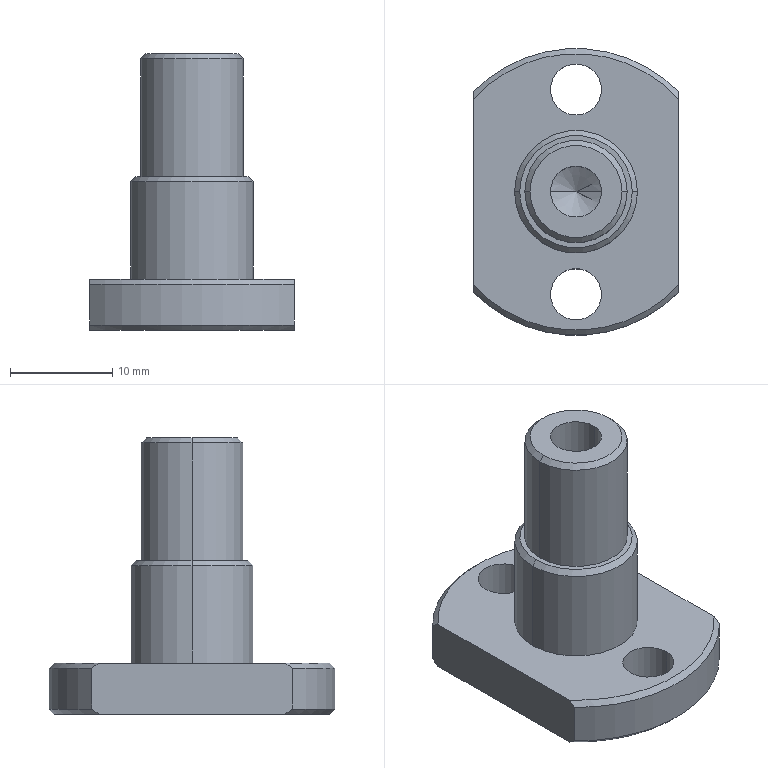Part | SolidWorks | features ICE 3, Chamfer 2, HoleWzd 2, Extrusion 1 | 1 solid | 28 faces | box 20 x 28 x 27 mm | volume 4092 mm3 | cylinder 12 | cone 10 | plane 6 | commonest cylinder face diameters 5 x6 10 x2 12 x2 28 x2
STEP:
#1=CARTESIAN_POINT('',(4.5,0.,22.));
#2=VERTEX_POINT('',#1);
#3=CARTESIAN_POINT('',(-4.5,0.,22.));
#4=VERTEX_POINT('',#3);
#5=CARTESIAN_POINT('',(0.,0.,22.));
#6=DIRECTION('',(0.,0.,1.));
#7=DIRECTION('',(1.,0.,0.));
#8=AXIS2_PLACEMENT_3D('',#5,#6,#7);
#9=CIRCLE('',#8,4.5);
#10=EDGE_CURVE('',#2,#4,#9,.T.);
#11=ORIENTED_EDGE('',*,*,#10,.F.);
#12=CARTESIAN_POINT('',(5.,0.,21.5));
#13=VERTEX_POINT('',#12);
#14=CARTESIAN_POINT('',(4.5,0.,22.));
#15=DIRECTION('',(0.7071,0.,-0.7071));
#16=VECTOR('',#15,1000.);
#17=LINE('',#14,#16);
#18=EDGE_CURVE('',#2,#13,#17,.T.);
#19=ORIENTED_EDGE('',*,*,#18,.T.);
#20=CARTESIAN_POINT('',(-5.,0.,21.5));
#21=VERTEX_POINT('',#20);
#22=CARTESIAN_POINT('',(0.,0.,21.5));
#23=DIRECTION('',(0.,0.,-1.));
#24=DIRECTION('',(1.,0.,0.));
#25=AXIS2_PLACEMENT_3D('',#22,#23,#24);
#26=CIRCLE('',#25,5.);
#27=EDGE_CURVE('',#21,#13,#26,.T.);
#28=ORIENTED_EDGE('',*,*,#27,.F.);
#29=CARTESIAN_POINT('',(-4.5,0.,22.));
#30=DIRECTION('',(-0.7071,0.,-0.7071));
#31=VECTOR('',#30,1000.);
#32=LINE('',#29,#31);
#33=EDGE_CURVE('',#4,#21,#32,.T.);
#34=ORIENTED_EDGE('',*,*,#33,.F.);
#35=EDGE_LOOP('',(#11,#19,#28,#34));
#36=FACE_OUTER_BOUND('',#35,.T.);
#37=CARTESIAN_POINT('',(0.,0.,22.));
#38=DIRECTION('',(0.,0.,-1.));
#39=DIRECTION('',(-1.,0.,0.));
#40=AXIS2_PLACEMENT_3D('',#37,#38,#39);
#41=CONICAL_SURFACE('',#40,4.5,0.7854);
#42=ADVANCED_FACE('',(#36),#41,.T.);
#43=CARTESIAN_POINT('',(5.5,0.,10.));
#44=VERTEX_POINT('',#43);
#45=CARTESIAN_POINT('',(-5.5,0.,10.));
#46=VERTEX_POINT('',#45);
#47=CARTESIAN_POINT('',(0.,0.,10.));
#48=DIRECTION('',(0.,0.,1.));
#49=DIRECTION('',(-1.,0.,0.));
#50=AXIS2_PLACEMENT_3D('',#47,#48,#49);
#51=CIRCLE('',#50,5.5);
#52=EDGE_CURVE('',#44,#46,#51,.T.);
#53=ORIENTED_EDGE('',*,*,#52,.F.);
#54=CARTESIAN_POINT('',(6.,0.,9.5));
#55=VERTEX_POINT('',#54);
#56=CARTESIAN_POINT('',(6.,0.,9.5));
#57=DIRECTION('',(0.7071,0.,-0.7071));
#58=VECTOR('',#57,1000.);
#59=LINE('',#56,#58);
#60=EDGE_CURVE('',#44,#55,#59,.T.);
#61=ORIENTED_EDGE('',*,*,#60,.T.);
#62=CARTESIAN_POINT('',(-6.,0.,9.5));
#63=VERTEX_POINT('',#62);
#64=CARTESIAN_POINT('',(0.,0.,9.5));
#65=DIRECTION('',(0.,0.,-1.));
#66=DIRECTION('',(-1.,0.,0.));
#67=AXIS2_PLACEMENT_3D('',#64,#65,#66);
#68=CIRCLE('',#67,6.);
#69=EDGE_CURVE('',#63,#55,#68,.T.);
#70=ORIENTED_EDGE('',*,*,#69,.F.);
#71=CARTESIAN_POINT('',(-6.,0.,9.5));
#72=DIRECTION('',(-0.7071,0.,-0.7071));
#73=VECTOR('',#72,1000.);
#74=LINE('',#71,#73);
#75=EDGE_CURVE('',#46,#63,#74,.T.);
#76=ORIENTED_EDGE('',*,*,#75,.F.);
#77=EDGE_LOOP('',(#53,#61,#70,#76));
#78=FACE_OUTER_BOUND('',#77,.T.);
#79=CARTESIAN_POINT('',(0.,0.,9.5));
#80=DIRECTION('',(0.,0.,-1.));
#81=DIRECTION('',(-1.,0.,0.));
#82=AXIS2_PLACEMENT_3D('',#79,#80,#81);
#83=CONICAL_SURFACE('',#82,6.,0.7854);
#84=ADVANCED_FACE('',(#78),#83,.T.);
#85=CARTESIAN_POINT('',(-2.5,0.,7.));
#86=VERTEX_POINT('',#85);
#87=CARTESIAN_POINT('',(2.5,0.,7.));
#88=VERTEX_POINT('',#87);
#89=CARTESIAN_POINT('',(0.,0.,7.));
#90=DIRECTION('',(0.,0.,1.));
#91=DIRECTION('',(1.,0.,0.));
#92=AXIS2_PLACEMENT_3D('',#89,#90,#91);
#93=CIRCLE('',#92,2.5);
#94=EDGE_CURVE('',#86,#88,#93,.T.);
#95=ORIENTED_EDGE('',*,*,#94,.F.);
#96=CARTESIAN_POINT('',(-2.5,0.,22.));
#97=VERTEX_POINT('',#96);
#98=CARTESIAN_POINT('',(-2.5,0.,22.));
#99=DIRECTION('',(0.,0.,1.));
#100=VECTOR('',#99,1000.);
#101=LINE('',#98,#100);
#102=EDGE_CURVE('',#86,#97,#101,.T.);
#103=ORIENTED_EDGE('',*,*,#102,.T.);
#104=CARTESIAN_POINT('',(2.5,0.,22.));
#105=VERTEX_POINT('',#104);
#106=CARTESIAN_POINT('',(0.,0.,22.));
#107=DIRECTION('',(0.,0.,1.));
#108=DIRECTION('',(1.,0.,0.));
#109=AXIS2_PLACEMENT_3D('',#106,#107,#108);
#110=CIRCLE('',#109,2.5);
#111=EDGE_CURVE('',#97,#105,#110,.T.);
#112=ORIENTED_EDGE('',*,*,#111,.T.);
#113=CARTESIAN_POINT('',(2.5,0.,22.));
#114=DIRECTION('',(0.,0.,1.));
#115=VECTOR('',#114,1000.);
#116=LINE('',#113,#115);
#117=EDGE_CURVE('',#88,#105,#116,.T.);
#118=ORIENTED_EDGE('',*,*,#117,.F.);
#119=EDGE_LOOP('',(#95,#103,#112,#118));
#120=FACE_OUTER_BOUND('',#119,.T.);
#121=CARTESIAN_POINT('',(0.,0.,22.));
#122=DIRECTION('',(0.,0.,1.));
#123=DIRECTION('',(1.,0.,0.));
#124=AXIS2_PLACEMENT_3D('',#121,#122,#123);
#125=CYLINDRICAL_SURFACE('',#124,2.5);
#126=ADVANCED_FACE('',(#120),#125,.F.);
#127=CARTESIAN_POINT('',(0.,0.,5.498));
#128=VERTEX_POINT('',#127);
#129=CARTESIAN_POINT('',(2.5,0.,7.));
#130=DIRECTION('',(0.8572,0.,0.515));
#131=VECTOR('',#130,1000.);
#132=LINE('',#129,#131);
#133=EDGE_CURVE('',#128,#88,#132,.T.);
#134=ORIENTED_EDGE('',*,*,#133,.F.);
#135=CARTESIAN_POINT('',(-2.5,0.,7.));
#136=DIRECTION('',(-0.8572,0.,0.515));
#137=VECTOR('',#136,1000.);
#138=LINE('',#135,#137);
#139=EDGE_CURVE('',#128,#86,#138,.T.);
#140=ORIENTED_EDGE('',*,*,#139,.T.);
#141=ORIENTED_EDGE('',*,*,#94,.T.);
#142=EDGE_LOOP('',(#134,#140,#141));
#143=FACE_OUTER_BOUND('',#142,.T.);
#144=CARTESIAN_POINT('',(0.,0.,7.));
#145=DIRECTION('',(0.,0.,1.));
#146=DIRECTION('',(1.,0.,0.));
#147=AXIS2_PLACEMENT_3D('',#144,#145,#146);
#148=CONICAL_SURFACE('',#147,2.5,1.03);
#149=ADVANCED_FACE('',(#143),#148,.F.);
#150=CARTESIAN_POINT('',(2.5,10.,-5.));
#151=VERTEX_POINT('',#150);
#152=CARTESIAN_POINT('',(-2.5,10.,-5.));
#153=VERTEX_POINT('',#152);
#154=CARTESIAN_POINT('',(0.,10.,-5.));
#155=DIRECTION('',(0.,0.,-1.));
#156=DIRECTION('',(-1.,0.,0.));
#157=AXIS2_PLACEMENT_3D('',#154,#155,#156);
#158=CIRCLE('',#157,2.5);
#159=EDGE_CURVE('',#151,#153,#158,.T.);
#160=ORIENTED_EDGE('',*,*,#159,.T.);
#161=CARTESIAN_POINT('',(-2.5,10.,0.));
#162=VERTEX_POINT('',#161);
#163=CARTESIAN_POINT('',(-2.5,10.,0.));
#164=DIRECTION('',(0.,0.,1.));
#165=VECTOR('',#164,1000.);
#166=LINE('',#163,#165);
#167=EDGE_CURVE('',#153,#162,#166,.T.);
#168=ORIENTED_EDGE('',*,*,#167,.T.);
#169=CARTESIAN_POINT('',(2.5,10.,0.));
#170=VERTEX_POINT('',#169);
#171=CARTESIAN_POINT('',(0.,10.,0.));
#172=DIRECTION('',(0.,0.,1.));
#173=DIRECTION('',(1.,0.,0.));
#174=AXIS2_PLACEMENT_3D('',#171,#172,#173);
#175=CIRCLE('',#174,2.5);
#176=EDGE_CURVE('',#162,#170,#175,.T.);
#177=ORIENTED_EDGE('',*,*,#176,.T.);
#178=CARTESIAN_POINT('',(2.5,10.,0.));
#179=DIRECTION('',(0.,0.,1.));
#180=VECTOR('',#179,1000.);
#181=LINE('',#178,#180);
#182=EDGE_CURVE('',#151,#170,#181,.T.);
#183=ORIENTED_EDGE('',*,*,#182,.F.);
#184=EDGE_LOOP('',(#160,#168,#177,#183));
#185=FACE_OUTER_BOUND('',#184,.T.);
#186=CARTESIAN_POINT('',(0.,10.,0.));
#187=DIRECTION('',(0.,0.,1.));
#188=DIRECTION('',(1.,0.,0.));
#189=AXIS2_PLACEMENT_3D('',#186,#187,#188);
#190=CYLINDRICAL_SURFACE('',#189,2.5);
#191=ADVANCED_FACE('',(#185),#190,.F.);
#192=CARTESIAN_POINT('',(2.5,-10.,-5.));
#193=VERTEX_POINT('',#192);
#194=CARTESIAN_POINT('',(-2.5,-10.,-5.));
#195=VERTEX_POINT('',#194);
#196=CARTESIAN_POINT('',(0.,-10.,-5.));
#197=DIRECTION('',(0.,0.,-1.));
#198=DIRECTION('',(-1.,0.,0.));
#199=AXIS2_PLACEMENT_3D('',#196,#197,#198);
#200=CIRCLE('',#199,2.5);
#201=EDGE_CURVE('',#193,#195,#200,.T.);
#202=ORIENTED_EDGE('',*,*,#201,.T.);
#203=CARTESIAN_POINT('',(-2.5,-10.,0.));
#204=VERTEX_POINT('',#203);
#205=CARTESIAN_POINT('',(-2.5,-10.,0.));
#206=DIRECTION('',(0.,0.,1.));
#207=VECTOR('',#206,1000.);
#208=LINE('',#205,#207);
#209=EDGE_CURVE('',#195,#204,#208,.T.);
#210=ORIENTED_EDGE('',*,*,#209,.T.);
#211=CARTESIAN_POINT('',(2.5,-10.,0.));
#212=VERTEX_POINT('',#211);
#213=CARTESIAN_POINT('',(0.,-10.,0.));
#214=DIRECTION('',(0.,0.,1.));
#215=DIRECTION('',(1.,0.,0.));
#216=AXIS2_PLACEMENT_3D('',#213,#214,#215);
#217=CIRCLE('',#216,2.5);
#218=EDGE_CURVE('',#204,#212,#217,.T.);
#219=ORIENTED_EDGE('',*,*,#218,.T.);
#220=CARTESIAN_POINT('',(2.5,-10.,0.));
#221=DIRECTION('',(0.,0.,1.));
#222=VECTOR('',#221,1000.);
#223=LINE('',#220,#222);
#224=EDGE_CURVE('',#193,#212,#223,.T.);
#225=ORIENTED_EDGE('',*,*,#224,.F.);
#226=EDGE_LOOP('',(#202,#210,#219,#225));
#227=FACE_OUTER_BOUND('',#226,.T.);
#228=CARTESIAN_POINT('',(0.,-10.,0.));
#229=DIRECTION('',(0.,0.,1.));
#230=DIRECTION('',(1.,0.,0.));
#231=AXIS2_PLACEMENT_3D('',#228,#229,#230);
#232=CYLINDRICAL_SURFACE('',#231,2.5);
#233=ADVANCED_FACE('',(#227),#232,.F.);
#234=ORIENTED_EDGE('',*,*,#69,.T.);
#235=CARTESIAN_POINT('',(6.,0.,0.));
#236=VERTEX_POINT('',#235);
#237=CARTESIAN_POINT('',(6.,0.,10.));
#238=DIRECTION('',(0.,0.,-1.));
#239=VECTOR('',#238,1000.);
#240=LINE('',#237,#239);
#241=EDGE_CURVE('',#55,#236,#240,.T.);
#242=ORIENTED_EDGE('',*,*,#241,.T.);
#243=CARTESIAN_POINT('',(-6.,0.,0.));
#244=VERTEX_POINT('',#243);
#245=CARTESIAN_POINT('',(0.,0.,0.));
#246=DIRECTION('',(0.,0.,-1.));
#247=DIRECTION('',(-1.,0.,0.));
#248=AXIS2_PLACEMENT_3D('',#245,#246,#247);
#249=CIRCLE('',#248,6.);
#250=EDGE_CURVE('',#244,#236,#249,.T.);
#251=ORIENTED_EDGE('',*,*,#250,.F.);
#252=CARTESIAN_POINT('',(-6.,0.,10.));
#253=DIRECTION('',(0.,0.,-1.));
#254=VECTOR('',#253,1000.);
#255=LINE('',#252,#254);
#256=EDGE_CURVE('',#63,#244,#255,.T.);
#257=ORIENTED_EDGE('',*,*,#256,.F.);
#258=EDGE_LOOP('',(#234,#242,#251,#257));
#259=FACE_OUTER_BOUND('',#258,.T.);
#260=CARTESIAN_POINT('',(0.,0.,10.));
#261=DIRECTION('',(0.,0.,-1.));
#262=DIRECTION('',(-1.,0.,0.));
#263=AXIS2_PLACEMENT_3D('',#260,#261,#262);
#264=CYLINDRICAL_SURFACE('',#263,6.);
#265=ADVANCED_FACE('',(#259),#264,.T.);
#266=ORIENTED_EDGE('',*,*,#27,.T.);
#267=CARTESIAN_POINT('',(5.,0.,10.));
#268=VERTEX_POINT('',#267);
#269=CARTESIAN_POINT('',(5.,0.,22.));
#270=DIRECTION('',(0.,0.,-1.));
#271=VECTOR('',#270,1000.);
#272=LINE('',#269,#271);
#273=EDGE_CURVE('',#13,#268,#272,.T.);
#274=ORIENTED_EDGE('',*,*,#273,.T.);
#275=CARTESIAN_POINT('',(-5.,0.,10.));
#276=VERTEX_POINT('',#275);
#277=CARTESIAN_POINT('',(0.,0.,10.));
#278=DIRECTION('',(0.,0.,-1.));
#279=DIRECTION('',(-1.,0.,0.));
#280=AXIS2_PLACEMENT_3D('',#277,#278,#279);
#281=CIRCLE('',#280,5.);
#282=EDGE_CURVE('',#276,#268,#281,.T.);
#283=ORIENTED_EDGE('',*,*,#282,.F.);
#284=CARTESIAN_POINT('',(-5.,0.,22.));
#285=DIRECTION('',(0.,0.,-1.));
#286=VECTOR('',#285,1000.);
#287=LINE('',#284,#286);
#288=EDGE_CURVE('',#21,#276,#287,.T.);
#289=ORIENTED_EDGE('',*,*,#288,.F.);
#290=EDGE_LOOP('',(#266,#274,#283,#289));
#291=FACE_OUTER_BOUND('',#290,.T.);
#292=CARTESIAN_POINT('',(0.,0.,22.));
#293=DIRECTION('',(0.,0.,-1.));
#294=DIRECTION('',(-1.,0.,0.));
#295=AXIS2_PLACEMENT_3D('',#292,#293,#294);
#296=CYLINDRICAL_SURFACE('',#295,5.);
#297=ADVANCED_FACE('',(#291),#296,.T.);
#298=CARTESIAN_POINT('',(10.,9.798,-4.5));
#299=VERTEX_POINT('',#298);
#300=CARTESIAN_POINT('',(10.,9.798,-0.5));
#301=VERTEX_POINT('',#300);
#302=CARTESIAN_POINT('',(10.,9.798,-5.));
#303=DIRECTION('',(0.,0.,1.));
#304=VECTOR('',#303,1000.);
#305=LINE('',#302,#304);
#306=EDGE_CURVE('',#299,#301,#305,.T.);
#307=ORIENTED_EDGE('',*,*,#306,.F.);
#308=CARTESIAN_POINT('',(-10.,9.798,-4.5));
#309=VERTEX_POINT('',#308);
#310=CARTESIAN_POINT('',(0.,0.,-4.5));
#311=DIRECTION('',(0.,0.,1.));
#312=DIRECTION('',(-1.,0.,0.));
#313=AXIS2_PLACEMENT_3D('',#310,#311,#312);
#314=CIRCLE('',#313,14.);
#315=EDGE_CURVE('',#299,#309,#314,.T.);
#316=ORIENTED_EDGE('',*,*,#315,.T.);
#317=CARTESIAN_POINT('',(-10.,9.798,-0.5));
#318=VERTEX_POINT('',#317);
#319=CARTESIAN_POINT('',(-10.,9.798,-5.));
#320=DIRECTION('',(0.,0.,-1.));
#321=VECTOR('',#320,1000.);
#322=LINE('',#319,#321);
#323=EDGE_CURVE('',#318,#309,#322,.T.);
#324=ORIENTED_EDGE('',*,*,#323,.F.);
#325=CARTESIAN_POINT('',(0.,0.,-0.5));
#326=DIRECTION('',(0.,0.,-1.));
#327=DIRECTION('',(-1.,0.,0.));
#328=AXIS2_PLACEMENT_3D('',#325,#326,#327);
#329=CIRCLE('',#328,14.);
#330=EDGE_CURVE('',#318,#301,#329,.T.);
#331=ORIENTED_EDGE('',*,*,#330,.T.);
#332=EDGE_LOOP('',(#307,#316,#324,#331));
#333=FACE_OUTER_BOUND('',#332,.T.);
#334=CARTESIAN_POINT('',(0.,0.,-5.));
#335=DIRECTION('',(0.,0.,1.));
#336=DIRECTION('',(1.,0.,0.));
#337=AXIS2_PLACEMENT_3D('',#334,#335,#336);
#338=CYLINDRICAL_SURFACE('',#337,14.);
#339=ADVANCED_FACE('',(#333),#338,.T.);
#340=CARTESIAN_POINT('',(-10.,-9.798,-4.5));
#341=VERTEX_POINT('',#340);
#342=CARTESIAN_POINT('',(-10.,-9.798,-0.5));
#343=VERTEX_POINT('',#342);
#344=CARTESIAN_POINT('',(-10.,-9.798,-5.));
#345=DIRECTION('',(0.,0.,1.));
#346=VECTOR('',#345,1000.);
#347=LINE('',#344,#346);
#348=EDGE_CURVE('',#341,#343,#347,.T.);
#349=ORIENTED_EDGE('',*,*,#348,.F.);
#350=CARTESIAN_POINT('',(10.,-9.798,-4.5));
#351=VERTEX_POINT('',#350);
#352=CARTESIAN_POINT('',(0.,0.,-4.5));
#353=DIRECTION('',(0.,0.,1.));
#354=DIRECTION('',(-1.,0.,0.));
#355=AXIS2_PLACEMENT_3D('',#352,#353,#354);
#356=CIRCLE('',#355,14.);
#357=EDGE_CURVE('',#341,#351,#356,.T.);
#358=ORIENTED_EDGE('',*,*,#357,.T.);
#359=CARTESIAN_POINT('',(10.,-9.798,-0.5));
#360=VERTEX_POINT('',#359);
#361=CARTESIAN_POINT('',(10.,-9.798,-5.));
#362=DIRECTION('',(0.,0.,-1.));
#363=VECTOR('',#362,1000.);
#364=LINE('',#361,#363);
#365=EDGE_CURVE('',#360,#351,#364,.T.);
#366=ORIENTED_EDGE('',*,*,#365,.F.);
#367=CARTESIAN_POINT('',(0.,0.,-0.5));
#368=DIRECTION('',(0.,0.,-1.));
#369=DIRECTION('',(-1.,0.,0.));
#370=AXIS2_PLACEMENT_3D('',#367,#368,#369);
#371=CIRCLE('',#370,14.);
#372=EDGE_CURVE('',#360,#343,#371,.T.);
#373=ORIENTED_EDGE('',*,*,#372,.T.);
#374=EDGE_LOOP('',(#349,#358,#366,#373));
#375=FACE_OUTER_BOUND('',#374,.T.);
#376=CARTESIAN_POINT('',(0.,0.,-5.));
#377=DIRECTION('',(0.,0.,1.));
#378=DIRECTION('',(1.,0.,0.));
#379=AXIS2_PLACEMENT_3D('',#376,#377,#378);
#380=CYLINDRICAL_SURFACE('',#379,14.);
#381=ADVANCED_FACE('',(#375),#380,.T.);
#382=ORIENTED_EDGE('',*,*,#159,.F.);
#383=CARTESIAN_POINT('',(0.,10.,-5.));
#384=DIRECTION('',(0.,0.,-1.));
#385=DIRECTION('',(-1.,0.,0.));
#386=AXIS2_PLACEMENT_3D('',#383,#384,#385);
#387=CIRCLE('',#386,2.5);
#388=EDGE_CURVE('',#153,#151,#387,.T.);
#389=ORIENTED_EDGE('',*,*,#388,.F.);
#390=EDGE_LOOP('',(#382,#389));
#391=FACE_BOUND('',#390,.T.);
#392=ORIENTED_EDGE('',*,*,#201,.F.);
#393=CARTESIAN_POINT('',(0.,-10.,-5.));
#394=DIRECTION('',(0.,0.,-1.));
#395=DIRECTION('',(-1.,0.,0.));
#396=AXIS2_PLACEMENT_3D('',#393,#394,#395);
#397=CIRCLE('',#396,2.5);
#398=EDGE_CURVE('',#195,#193,#397,.T.);
#399=ORIENTED_EDGE('',*,*,#398,.F.);
#400=EDGE_LOOP('',(#392,#399));
#401=FACE_BOUND('',#400,.T.);
#402=CARTESIAN_POINT('',(10.,9.069,-5.));
#403=VERTEX_POINT('',#402);
#404=CARTESIAN_POINT('',(10.,-9.069,-5.));
#405=VERTEX_POINT('',#404);
#406=CARTESIAN_POINT('',(10.,18.644,-5.));
#407=DIRECTION('',(0.,-1.,0.));
#408=VECTOR('',#407,1000.);
#409=LINE('',#406,#408);
#410=EDGE_CURVE('',#403,#405,#409,.T.);
#411=ORIENTED_EDGE('',*,*,#410,.T.);
#412=CARTESIAN_POINT('',(-10.,-9.069,-5.));
#413=VERTEX_POINT('',#412);
#414=CARTESIAN_POINT('',(0.,0.,-5.));
#415=DIRECTION('',(0.,0.,-1.));
#416=DIRECTION('',(-1.,0.,0.));
#417=AXIS2_PLACEMENT_3D('',#414,#415,#416);
#418=CIRCLE('',#417,13.5);
#419=EDGE_CURVE('',#405,#413,#418,.T.);
#420=ORIENTED_EDGE('',*,*,#419,.T.);
#421=CARTESIAN_POINT('',(-10.,9.069,-5.));
#422=VERTEX_POINT('',#421);
#423=CARTESIAN_POINT('',(-10.,18.644,-5.));
#424=DIRECTION('',(0.,1.,0.));
#425=VECTOR('',#424,1000.);
#426=LINE('',#423,#425);
#427=EDGE_CURVE('',#413,#422,#426,.T.);
#428=ORIENTED_EDGE('',*,*,#427,.T.);
#429=CARTESIAN_POINT('',(0.,0.,-5.));
#430=DIRECTION('',(0.,0.,-1.));
#431=DIRECTION('',(-1.,0.,0.));
#432=AXIS2_PLACEMENT_3D('',#429,#430,#431);
#433=CIRCLE('',#432,13.5);
#434=EDGE_CURVE('',#422,#403,#433,.T.);
#435=ORIENTED_EDGE('',*,*,#434,.T.);
#436=EDGE_LOOP('',(#411,#420,#428,#435));
#437=FACE_OUTER_BOUND('',#436,.T.);
#438=CARTESIAN_POINT('',(0.,0.,-5.));
#439=DIRECTION('',(0.,0.,-1.));
#440=DIRECTION('',(-1.,0.,0.));
#441=AXIS2_PLACEMENT_3D('',#438,#439,#440);
#442=PLANE('',#441);
#443=ADVANCED_FACE('',(#391,#401,#437),#442,.T.);
#444=CARTESIAN_POINT('',(0.,10.,0.));
#445=DIRECTION('',(0.,0.,1.));
#446=DIRECTION('',(1.,0.,0.));
#447=AXIS2_PLACEMENT_3D('',#444,#445,#446);
#448=CIRCLE('',#447,2.5);
#449=EDGE_CURVE('',#170,#162,#448,.T.);
#450=ORIENTED_EDGE('',*,*,#449,.F.);
#451=ORIENTED_EDGE('',*,*,#176,.F.);
#452=EDGE_LOOP('',(#450,#451));
#453=FACE_BOUND('',#452,.T.);
#454=CARTESIAN_POINT('',(0.,-10.,0.));
#455=DIRECTION('',(0.,0.,1.));
#456=DIRECTION('',(1.,0.,0.));
#457=AXIS2_PLACEMENT_3D('',#454,#455,#456);
#458=CIRCLE('',#457,2.5);
#459=EDGE_CURVE('',#212,#204,#458,.T.);
#460=ORIENTED_EDGE('',*,*,#459,.F.);
#461=ORIENTED_EDGE('',*,*,#218,.F.);
#462=EDGE_LOOP('',(#460,#461));
#463=FACE_BOUND('',#462,.T.);
#464=ORIENTED_EDGE('',*,*,#250,.T.);
#465=CARTESIAN_POINT('',(0.,0.,0.));
#466=DIRECTION('',(0.,0.,-1.));
#467=DIRECTION('',(-1.,0.,0.));
#468=AXIS2_PLACEMENT_3D('',#465,#466,#467);
#469=CIRCLE('',#468,6.);
#470=EDGE_CURVE('',#236,#244,#469,.T.);
#471=ORIENTED_EDGE('',*,*,#470,.T.);
#472=EDGE_LOOP('',(#464,#471));
#473=FACE_BOUND('',#472,.T.);
#474=CARTESIAN_POINT('',(10.,9.069,0.));
#475=VERTEX_POINT('',#474);
#476=CARTESIAN_POINT('',(10.,-9.069,0.));
#477=VERTEX_POINT('',#476);
#478=CARTESIAN_POINT('',(10.,0.,0.));
#479=DIRECTION('',(0.,-1.,0.));
#480=VECTOR('',#479,1000.);
#481=LINE('',#478,#480);
#482=EDGE_CURVE('',#475,#477,#481,.T.);
#483=ORIENTED_EDGE('',*,*,#482,.F.);
#484=CARTESIAN_POINT('',(-10.,9.069,0.));
#485=VERTEX_POINT('',#484);
#486=CARTESIAN_POINT('',(0.,0.,0.));
#487=DIRECTION('',(0.,0.,1.));
#488=DIRECTION('',(-1.,0.,0.));
#489=AXIS2_PLACEMENT_3D('',#486,#487,#488);
#490=CIRCLE('',#489,13.5);
#491=EDGE_CURVE('',#475,#485,#490,.T.);
#492=ORIENTED_EDGE('',*,*,#491,.T.);
#493=CARTESIAN_POINT('',(-10.,-9.069,0.));
#494=VERTEX_POINT('',#493);
#495=CARTESIAN_POINT('',(-10.,0.,0.));
#496=DIRECTION('',(0.,1.,0.));
#497=VECTOR('',#496,1000.);
#498=LINE('',#495,#497);
#499=EDGE_CURVE('',#494,#485,#498,.T.);
#500=ORIENTED_EDGE('',*,*,#499,.F.);
#501=CARTESIAN_POINT('',(0.,0.,0.));
#502=DIRECTION('',(0.,0.,1.));
#503=DIRECTION('',(-1.,0.,0.));
#504=AXIS2_PLACEMENT_3D('',#501,#502,#503);
#505=CIRCLE('',#504,13.5);
#506=EDGE_CURVE('',#494,#477,#505,.T.);
#507=ORIENTED_EDGE('',*,*,#506,.T.);
#508=EDGE_LOOP('',(#483,#492,#500,#507));
#509=FACE_OUTER_BOUND('',#508,.T.);
#510=CARTESIAN_POINT('',(0.,0.,0.));
#511=DIRECTION('',(0.,0.,-1.));
#512=DIRECTION('',(-1.,0.,0.));
#513=AXIS2_PLACEMENT_3D('',#510,#511,#512);
#514=PLANE('',#513);
#515=ADVANCED_FACE('',(#453,#463,#473,#509),#514,.F.);
#516=ORIENTED_EDGE('',*,*,#273,.F.);
#517=CARTESIAN_POINT('',(0.,0.,21.5));
#518=DIRECTION('',(0.,0.,-1.));
#519=DIRECTION('',(1.,0.,0.));
#520=AXIS2_PLACEMENT_3D('',#517,#518,#519);
#521=CIRCLE('',#520,5.);
#522=EDGE_CURVE('',#13,#21,#521,.T.);
#523=ORIENTED_EDGE('',*,*,#522,.T.);
#524=ORIENTED_EDGE('',*,*,#288,.T.);
#525=CARTESIAN_POINT('',(0.,0.,10.));
#526=DIRECTION('',(0.,0.,-1.));
#527=DIRECTION('',(-1.,0.,0.));
#528=AXIS2_PLACEMENT_3D('',#525,#526,#527);
#529=CIRCLE('',#528,5.);
#530=EDGE_CURVE('',#268,#276,#529,.T.);
#531=ORIENTED_EDGE('',*,*,#530,.F.);
#532=EDGE_LOOP('',(#516,#523,#524,#531));
#533=FACE_OUTER_BOUND('',#532,.T.);
#534=CARTESIAN_POINT('',(0.,0.,22.));
#535=DIRECTION('',(0.,0.,-1.));
#536=DIRECTION('',(-1.,0.,0.));
#537=AXIS2_PLACEMENT_3D('',#534,#535,#536);
#538=CYLINDRICAL_SURFACE('',#537,5.);
#539=ADVANCED_FACE('',(#533),#538,.T.);
#540=CARTESIAN_POINT('',(0.,0.,22.));
#541=DIRECTION('',(0.,0.,1.));
#542=DIRECTION('',(1.,0.,0.));
#543=AXIS2_PLACEMENT_3D('',#540,#541,#542);
#544=CIRCLE('',#543,4.5);
#545=EDGE_CURVE('',#4,#2,#544,.T.);
#546=ORIENTED_EDGE('',*,*,#545,.T.);
#547=ORIENTED_EDGE('',*,*,#10,.T.);
#548=EDGE_LOOP('',(#546,#547));
#549=FACE_OUTER_BOUND('',#548,.T.);
#550=CARTESIAN_POINT('',(0.,0.,22.));
#551=DIRECTION('',(0.,0.,1.));
#552=DIRECTION('',(1.,0.,0.));
#553=AXIS2_PLACEMENT_3D('',#550,#551,#552);
#554=CIRCLE('',#553,2.5);
#555=EDGE_CURVE('',#105,#97,#554,.T.);
#556=ORIENTED_EDGE('',*,*,#555,.F.);
#557=ORIENTED_EDGE('',*,*,#111,.F.);
#558=EDGE_LOOP('',(#556,#557));
#559=FACE_BOUND('',#558,.T.);
#560=CARTESIAN_POINT('',(0.,0.,22.));
#561=DIRECTION('',(0.,0.,1.));
#562=DIRECTION('',(1.,0.,0.));
#563=AXIS2_PLACEMENT_3D('',#560,#561,#562);
#564=PLANE('',#563);
#565=ADVANCED_FACE('',(#549,#559),#564,.T.);
#566=CARTESIAN_POINT('',(0.,0.,10.));
#567=DIRECTION('',(0.,0.,1.));
#568=DIRECTION('',(-1.,0.,0.));
#569=AXIS2_PLACEMENT_3D('',#566,#567,#568);
#570=CIRCLE('',#569,5.5);
#571=EDGE_CURVE('',#46,#44,#570,.T.);
#572=ORIENTED_EDGE('',*,*,#571,.T.);
#573=ORIENTED_EDGE('',*,*,#52,.T.);
#574=EDGE_LOOP('',(#572,#573));
#575=FACE_OUTER_BOUND('',#574,.T.);
#576=ORIENTED_EDGE('',*,*,#282,.T.);
#577=ORIENTED_EDGE('',*,*,#530,.T.);
#578=EDGE_LOOP('',(#576,#577));
#579=FACE_BOUND('',#578,.T.);
#580=CARTESIAN_POINT('',(0.,0.,10.));
#581=DIRECTION('',(0.,0.,-1.));
#582=DIRECTION('',(-1.,0.,0.));
#583=AXIS2_PLACEMENT_3D('',#580,#581,#582);
#584=PLANE('',#583);
#585=ADVANCED_FACE('',(#575,#579),#584,.F.);
#586=ORIENTED_EDGE('',*,*,#241,.F.);
#587=CARTESIAN_POINT('',(0.,0.,9.5));
#588=DIRECTION('',(0.,0.,-1.));
#589=DIRECTION('',(-1.,0.,0.));
#590=AXIS2_PLACEMENT_3D('',#587,#588,#589);
#591=CIRCLE('',#590,6.);
#592=EDGE_CURVE('',#55,#63,#591,.T.);
#593=ORIENTED_EDGE('',*,*,#592,.T.);
#594=ORIENTED_EDGE('',*,*,#256,.T.);
#595=ORIENTED_EDGE('',*,*,#470,.F.);
#596=EDGE_LOOP('',(#586,#593,#594,#595));
#597=FACE_OUTER_BOUND('',#596,.T.);
#598=CARTESIAN_POINT('',(0.,0.,10.));
#599=DIRECTION('',(0.,0.,-1.));
#600=DIRECTION('',(-1.,0.,0.));
#601=AXIS2_PLACEMENT_3D('',#598,#599,#600);
#602=CYLINDRICAL_SURFACE('',#601,6.);
#603=ADVANCED_FACE('',(#597),#602,.T.);
#604=ORIENTED_EDGE('',*,*,#427,.F.);
#605=CARTESIAN_POINT('',(-10.,-9.069,-5.));
#606=CARTESIAN_POINT('',(-10.,-9.314,-4.836));
#607=CARTESIAN_POINT('',(-10.,-9.557,-4.669));
#608=CARTESIAN_POINT('',(-10.,-9.798,-4.5));
#609=B_SPLINE_CURVE_WITH_KNOTS('',3,(#605,#606,#607,#608),.UNSPECIFIED.,.F.,.F.,(4,4),(0.,0.0008838),.UNSPECIFIED.);
#610=EDGE_CURVE('',#413,#341,#609,.T.);
#611=ORIENTED_EDGE('',*,*,#610,.T.);
#612=ORIENTED_EDGE('',*,*,#348,.T.);
#613=CARTESIAN_POINT('',(-10.,-9.798,-0.5));
#614=CARTESIAN_POINT('',(-10.,-9.557,-0.3311));
#615=CARTESIAN_POINT('',(-10.,-9.314,-0.1643));
#616=CARTESIAN_POINT('',(-10.,-9.069,0.));
#617=B_SPLINE_CURVE_WITH_KNOTS('',3,(#613,#614,#615,#616),.UNSPECIFIED.,.F.,.F.,(4,4),(0.,0.0008838),.UNSPECIFIED.);
#618=EDGE_CURVE('',#343,#494,#617,.T.);
#619=ORIENTED_EDGE('',*,*,#618,.T.);
#620=ORIENTED_EDGE('',*,*,#499,.T.);
#621=CARTESIAN_POINT('',(-10.,9.069,0.));
#622=CARTESIAN_POINT('',(-10.,9.314,-0.1643));
#623=CARTESIAN_POINT('',(-10.,9.557,-0.3311));
#624=CARTESIAN_POINT('',(-10.,9.798,-0.5));
#625=B_SPLINE_CURVE_WITH_KNOTS('',3,(#621,#622,#623,#624),.UNSPECIFIED.,.F.,.F.,(4,4),(0.,0.0008838),.UNSPECIFIED.);
#626=EDGE_CURVE('',#485,#318,#625,.T.);
#627=ORIENTED_EDGE('',*,*,#626,.T.);
#628=ORIENTED_EDGE('',*,*,#323,.T.);
#629=CARTESIAN_POINT('',(-10.,9.798,-4.5));
#630=CARTESIAN_POINT('',(-10.,9.557,-4.669));
#631=CARTESIAN_POINT('',(-10.,9.314,-4.836));
#632=CARTESIAN_POINT('',(-10.,9.069,-5.));
#633=B_SPLINE_CURVE_WITH_KNOTS('',3,(#629,#630,#631,#632),.UNSPECIFIED.,.F.,.F.,(4,4),(0.,0.0008838),.UNSPECIFIED.);
#634=EDGE_CURVE('',#309,#422,#633,.T.);
#635=ORIENTED_EDGE('',*,*,#634,.T.);
#636=EDGE_LOOP('',(#604,#611,#612,#619,#620,#627,#628,#635));
#637=FACE_OUTER_BOUND('',#636,.T.);
#638=CARTESIAN_POINT('',(-10.,18.644,0.));
#639=DIRECTION('',(-1.,0.,0.));
#640=DIRECTION('',(0.,-1.,0.));
#641=AXIS2_PLACEMENT_3D('',#638,#639,#640);
#642=PLANE('',#641);
#643=ADVANCED_FACE('',(#637),#642,.T.);
#644=ORIENTED_EDGE('',*,*,#365,.T.);
#645=CARTESIAN_POINT('',(10.,-9.798,-4.5));
#646=CARTESIAN_POINT('',(10.,-9.557,-4.669));
#647=CARTESIAN_POINT('',(10.,-9.314,-4.836));
#648=CARTESIAN_POINT('',(10.,-9.069,-5.));
#649=B_SPLINE_CURVE_WITH_KNOTS('',3,(#645,#646,#647,#648),.UNSPECIFIED.,.F.,.F.,(4,4),(0.,0.0008838),.UNSPECIFIED.);
#650=EDGE_CURVE('',#351,#405,#649,.T.);
#651=ORIENTED_EDGE('',*,*,#650,.T.);
#652=ORIENTED_EDGE('',*,*,#410,.F.);
#653=CARTESIAN_POINT('',(10.,9.069,-5.));
#654=CARTESIAN_POINT('',(10.,9.314,-4.836));
#655=CARTESIAN_POINT('',(10.,9.557,-4.669));
#656=CARTESIAN_POINT('',(10.,9.798,-4.5));
#657=B_SPLINE_CURVE_WITH_KNOTS('',3,(#653,#654,#655,#656),.UNSPECIFIED.,.F.,.F.,(4,4),(0.,0.0008838),.UNSPECIFIED.);
#658=EDGE_CURVE('',#403,#299,#657,.T.);
#659=ORIENTED_EDGE('',*,*,#658,.T.);
#660=ORIENTED_EDGE('',*,*,#306,.T.);
#661=CARTESIAN_POINT('',(10.,9.798,-0.5));
#662=CARTESIAN_POINT('',(10.,9.557,-0.3311));
#663=CARTESIAN_POINT('',(10.,9.314,-0.1643));
#664=CARTESIAN_POINT('',(10.,9.069,0.));
#665=B_SPLINE_CURVE_WITH_KNOTS('',3,(#661,#662,#663,#664),.UNSPECIFIED.,.F.,.F.,(4,4),(0.,0.0008838),.UNSPECIFIED.);
#666=EDGE_CURVE('',#301,#475,#665,.T.);
#667=ORIENTED_EDGE('',*,*,#666,.T.);
#668=ORIENTED_EDGE('',*,*,#482,.T.);
#669=CARTESIAN_POINT('',(10.,-9.069,0.));
#670=CARTESIAN_POINT('',(10.,-9.314,-0.1643));
#671=CARTESIAN_POINT('',(10.,-9.557,-0.3311));
#672=CARTESIAN_POINT('',(10.,-9.798,-0.5));
#673=B_SPLINE_CURVE_WITH_KNOTS('',3,(#669,#670,#671,#672),.UNSPECIFIED.,.F.,.F.,(4,4),(0.,0.0008838),.UNSPECIFIED.);
#674=EDGE_CURVE('',#477,#360,#673,.T.);
#675=ORIENTED_EDGE('',*,*,#674,.T.);
#676=EDGE_LOOP('',(#644,#651,#652,#659,#660,#667,#668,#675));
#677=FACE_OUTER_BOUND('',#676,.T.);
#678=CARTESIAN_POINT('',(10.,18.644,0.));
#679=DIRECTION('',(1.,0.,0.));
#680=DIRECTION('',(0.,1.,0.));
#681=AXIS2_PLACEMENT_3D('',#678,#679,#680);
#682=PLANE('',#681);
#683=ADVANCED_FACE('',(#677),#682,.T.);
#684=ORIENTED_EDGE('',*,*,#209,.F.);
#685=ORIENTED_EDGE('',*,*,#398,.T.);
#686=ORIENTED_EDGE('',*,*,#224,.T.);
#687=ORIENTED_EDGE('',*,*,#459,.T.);
#688=EDGE_LOOP('',(#684,#685,#686,#687));
#689=FACE_OUTER_BOUND('',#688,.T.);
#690=CARTESIAN_POINT('',(0.,-10.,0.));
#691=DIRECTION('',(0.,0.,1.));
#692=DIRECTION('',(1.,0.,0.));
#693=AXIS2_PLACEMENT_3D('',#690,#691,#692);
#694=CYLINDRICAL_SURFACE('',#693,2.5);
#695=ADVANCED_FACE('',(#689),#694,.F.);
#696=ORIENTED_EDGE('',*,*,#167,.F.);
#697=ORIENTED_EDGE('',*,*,#388,.T.);
#698=ORIENTED_EDGE('',*,*,#182,.T.);
#699=ORIENTED_EDGE('',*,*,#449,.T.);
#700=EDGE_LOOP('',(#696,#697,#698,#699));
#701=FACE_OUTER_BOUND('',#700,.T.);
#702=CARTESIAN_POINT('',(0.,10.,0.));
#703=DIRECTION('',(0.,0.,1.));
#704=DIRECTION('',(1.,0.,0.));
#705=AXIS2_PLACEMENT_3D('',#702,#703,#704);
#706=CYLINDRICAL_SURFACE('',#705,2.5);
#707=ADVANCED_FACE('',(#701),#706,.F.);
#708=ORIENTED_EDGE('',*,*,#139,.F.);
#709=ORIENTED_EDGE('',*,*,#133,.T.);
#710=CARTESIAN_POINT('',(0.,0.,7.));
#711=DIRECTION('',(0.,0.,1.));
#712=DIRECTION('',(1.,0.,0.));
#713=AXIS2_PLACEMENT_3D('',#710,#711,#712);
#714=CIRCLE('',#713,2.5);
#715=EDGE_CURVE('',#88,#86,#714,.T.);
#716=ORIENTED_EDGE('',*,*,#715,.T.);
#717=EDGE_LOOP('',(#708,#709,#716));
#718=FACE_OUTER_BOUND('',#717,.T.);
#719=CARTESIAN_POINT('',(0.,0.,7.));
#720=DIRECTION('',(0.,0.,1.));
#721=DIRECTION('',(1.,0.,0.));
#722=AXIS2_PLACEMENT_3D('',#719,#720,#721);
#723=CONICAL_SURFACE('',#722,2.5,1.03);
#724=ADVANCED_FACE('',(#718),#723,.F.);
#725=ORIENTED_EDGE('',*,*,#102,.F.);
#726=ORIENTED_EDGE('',*,*,#715,.F.);
#727=ORIENTED_EDGE('',*,*,#117,.T.);
#728=ORIENTED_EDGE('',*,*,#555,.T.);
#729=EDGE_LOOP('',(#725,#726,#727,#728));
#730=FACE_OUTER_BOUND('',#729,.T.);
#731=CARTESIAN_POINT('',(0.,0.,22.));
#732=DIRECTION('',(0.,0.,1.));
#733=DIRECTION('',(1.,0.,0.));
#734=AXIS2_PLACEMENT_3D('',#731,#732,#733);
#735=CYLINDRICAL_SURFACE('',#734,2.5);
#736=ADVANCED_FACE('',(#730),#735,.F.);
#737=ORIENTED_EDGE('',*,*,#60,.F.);
#738=ORIENTED_EDGE('',*,*,#571,.F.);
#739=ORIENTED_EDGE('',*,*,#75,.T.);
#740=ORIENTED_EDGE('',*,*,#592,.F.);
#741=EDGE_LOOP('',(#737,#738,#739,#740));
#742=FACE_OUTER_BOUND('',#741,.T.);
#743=CARTESIAN_POINT('',(0.,0.,9.5));
#744=DIRECTION('',(0.,0.,-1.));
#745=DIRECTION('',(-1.,0.,0.));
#746=AXIS2_PLACEMENT_3D('',#743,#744,#745);
#747=CONICAL_SURFACE('',#746,6.,0.7854);
#748=ADVANCED_FACE('',(#742),#747,.T.);
#749=ORIENTED_EDGE('',*,*,#18,.F.);
#750=ORIENTED_EDGE('',*,*,#545,.F.);
#751=ORIENTED_EDGE('',*,*,#33,.T.);
#752=ORIENTED_EDGE('',*,*,#522,.F.);
#753=EDGE_LOOP('',(#749,#750,#751,#752));
#754=FACE_OUTER_BOUND('',#753,.T.);
#755=CARTESIAN_POINT('',(0.,0.,22.));
#756=DIRECTION('',(0.,0.,-1.));
#757=DIRECTION('',(-1.,0.,0.));
#758=AXIS2_PLACEMENT_3D('',#755,#756,#757);
#759=CONICAL_SURFACE('',#758,4.5,0.7854);
#760=ADVANCED_FACE('',(#754),#759,.T.);
#761=ORIENTED_EDGE('',*,*,#650,.F.);
#762=ORIENTED_EDGE('',*,*,#357,.F.);
#763=ORIENTED_EDGE('',*,*,#610,.F.);
#764=ORIENTED_EDGE('',*,*,#419,.F.);
#765=EDGE_LOOP('',(#761,#762,#763,#764));
#766=FACE_OUTER_BOUND('',#765,.T.);
#767=CARTESIAN_POINT('',(0.,0.,-5.));
#768=DIRECTION('',(0.,0.,1.));
#769=DIRECTION('',(1.,0.,0.));
#770=AXIS2_PLACEMENT_3D('',#767,#768,#769);
#771=CONICAL_SURFACE('',#770,13.5,0.7854);
#772=ADVANCED_FACE('',(#766),#771,.T.);
#773=ORIENTED_EDGE('',*,*,#634,.F.);
#774=ORIENTED_EDGE('',*,*,#315,.F.);
#775=ORIENTED_EDGE('',*,*,#658,.F.);
#776=ORIENTED_EDGE('',*,*,#434,.F.);
#777=EDGE_LOOP('',(#773,#774,#775,#776));
#778=FACE_OUTER_BOUND('',#777,.T.);
#779=CARTESIAN_POINT('',(0.,0.,-5.));
#780=DIRECTION('',(0.,0.,1.));
#781=DIRECTION('',(1.,0.,0.));
#782=AXIS2_PLACEMENT_3D('',#779,#780,#781);
#783=CONICAL_SURFACE('',#782,13.5,0.7854);
#784=ADVANCED_FACE('',(#778),#783,.T.);
#785=ORIENTED_EDGE('',*,*,#626,.F.);
#786=ORIENTED_EDGE('',*,*,#491,.F.);
#787=ORIENTED_EDGE('',*,*,#666,.F.);
#788=ORIENTED_EDGE('',*,*,#330,.F.);
#789=EDGE_LOOP('',(#785,#786,#787,#788));
#790=FACE_OUTER_BOUND('',#789,.T.);
#791=CARTESIAN_POINT('',(0.,0.,-0.5));
#792=DIRECTION('',(0.,0.,-1.));
#793=DIRECTION('',(-1.,0.,0.));
#794=AXIS2_PLACEMENT_3D('',#791,#792,#793);
#795=CONICAL_SURFACE('',#794,14.,0.7854);
#796=ADVANCED_FACE('',(#790),#795,.T.);
#797=ORIENTED_EDGE('',*,*,#674,.F.);
#798=ORIENTED_EDGE('',*,*,#506,.F.);
#799=ORIENTED_EDGE('',*,*,#618,.F.);
#800=ORIENTED_EDGE('',*,*,#372,.F.);
#801=EDGE_LOOP('',(#797,#798,#799,#800));
#802=FACE_OUTER_BOUND('',#801,.T.);
#803=CARTESIAN_POINT('',(0.,0.,-0.5));
#804=DIRECTION('',(0.,0.,-1.));
#805=DIRECTION('',(-1.,0.,0.));
#806=AXIS2_PLACEMENT_3D('',#803,#804,#805);
#807=CONICAL_SURFACE('',#806,14.,0.7854);
#808=ADVANCED_FACE('',(#802),#807,.T.);
#809=CLOSED_SHELL('',(#42,#84,#126,#149,#191,#233,#265,#297,#339,#381,#443,#515,#539,#565,#585,#603,#643,#683,#695,#707,#724,#736,#748,#760,#772,#784,#796,#808));
#810=MANIFOLD_SOLID_BREP('',#809);
#811=CARTESIAN_POINT('',(0.,0.,0.));
#812=DIRECTION('',(0.,0.,1.));
#813=DIRECTION('',(1.,0.,0.));
#814=AXIS2_PLACEMENT_3D('',#811,#812,#813);
#815=(LENGTH_UNIT()NAMED_UNIT(*)SI_UNIT(.MILLI.,.METRE.));
#816=UNCERTAINTY_MEASURE_WITH_UNIT(LENGTH_MEASURE(0.00001),#815,'','');
#817=(NAMED_UNIT(*)PLANE_ANGLE_UNIT()SI_UNIT($,.RADIAN.));
#818=(NAMED_UNIT(*)SI_UNIT($,.STERADIAN.)SOLID_ANGLE_UNIT());
#819=(GEOMETRIC_REPRESENTATION_CONTEXT(3)GLOBAL_UNCERTAINTY_ASSIGNED_CONTEXT((#816))GLOBAL_UNIT_ASSIGNED_CONTEXT((#815,#817,#818))REPRESENTATION_CONTEXT('',''));
#820=ADVANCED_BREP_SHAPE_REPRESENTATION('',(#810,#814),#819);